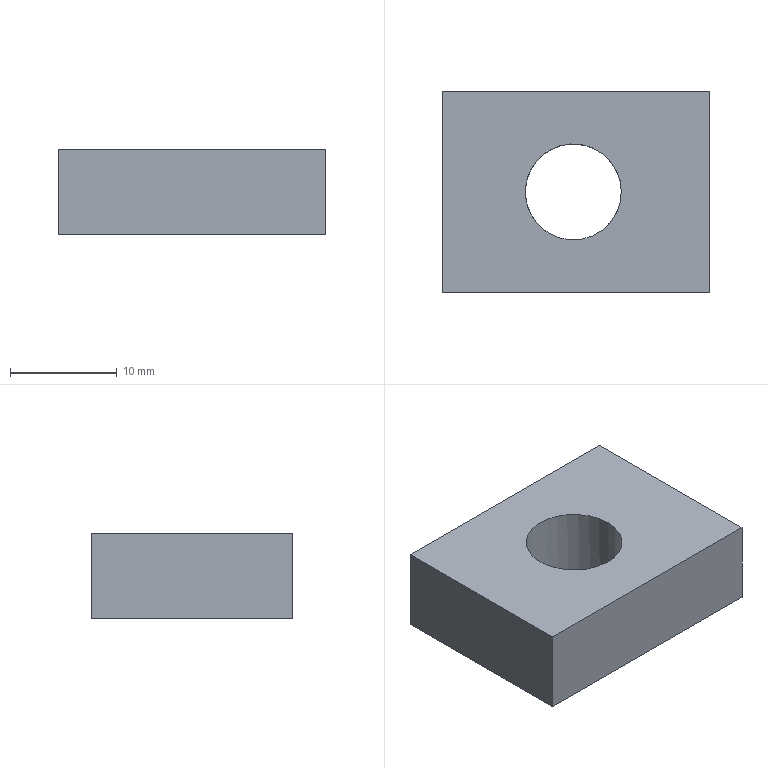Part | STEP file | gslz 2016.10.28-10_id1158_x_t | 1 solid | 7 faces | box 25.1 x 18.9 x 8 mm | volume 3286 mm3 | plane 6 | cylinder 1 | commonest cylinder face diameters 9 x1
STEP:
#1=CARTESIAN_POINT('',(0.,0.,0.));
#2=DIRECTION('',(0.,0.,1.));
#3=DIRECTION('',(1.,0.,0.));
#4=AXIS2_PLACEMENT_3D('',#1,#2,#3);
#5=CARTESIAN_POINT('',(-705.8,671.25,110.));
#6=VERTEX_POINT('',#5);
#7=CARTESIAN_POINT('',(-705.8,690.15,110.));
#8=VERTEX_POINT('',#7);
#9=CARTESIAN_POINT('',(-705.8,701.15,110.));
#10=DIRECTION('',(0.,1.,0.));
#11=VECTOR('',#10,1.);
#12=LINE('',#9,#11);
#13=CARTESIAN_POINT('',(-705.8,701.15,110.));
#14=DIRECTION('',(1.,0.,0.));
#15=DIRECTION('',(0.,0.,1.));
#16=AXIS2_PLACEMENT_3D('',#13,#14,#15);
#17=PLANE('',#16);
#18=CARTESIAN_POINT('',(0.,0.));
#19=DIRECTION('',(0.,-1.));
#20=VECTOR('',#19,1.);
#21=LINE('',#18,#20);
#22=(GEOMETRIC_REPRESENTATION_CONTEXT(2)PARAMETRIC_REPRESENTATION_CONTEXT()REPRESENTATION_CONTEXT('',''));
#23=DEFINITIONAL_REPRESENTATION('',(#21),#22);
#24=PCURVE('',#17,#23);
#25=CARTESIAN_POINT('',(-702.3,701.15,110.));
#26=DIRECTION('',(0.,0.,-1.));
#27=DIRECTION('',(1.,0.,0.));
#28=AXIS2_PLACEMENT_3D('',#25,#26,#27);
#29=PLANE('',#28);
#30=CARTESIAN_POINT('',(-3.5,0.));
#31=DIRECTION('',(0.,-1.));
#32=VECTOR('',#31,1.);
#33=LINE('',#30,#32);
#34=(GEOMETRIC_REPRESENTATION_CONTEXT(2)PARAMETRIC_REPRESENTATION_CONTEXT()REPRESENTATION_CONTEXT('',''));
#35=DEFINITIONAL_REPRESENTATION('',(#33),#34);
#36=PCURVE('',#29,#35);
#37=SURFACE_CURVE('',#12,(#24,#36),.PCURVE_S1.);
#38=EDGE_CURVE('',#6,#8,#37,.T.);
#39=ORIENTED_EDGE('',*,*,#38,.T.);
#40=CARTESIAN_POINT('',(-705.8,690.15,102.));
#41=VERTEX_POINT('',#40);
#42=CARTESIAN_POINT('',(-705.8,690.15,35.163));
#43=DIRECTION('',(0.,0.,-1.));
#44=VECTOR('',#43,1.);
#45=LINE('',#42,#44);
#46=CARTESIAN_POINT('',(-74.837,11.));
#47=DIRECTION('',(-1.,0.));
#48=VECTOR('',#47,1.);
#49=LINE('',#46,#48);
#50=(GEOMETRIC_REPRESENTATION_CONTEXT(2)PARAMETRIC_REPRESENTATION_CONTEXT()REPRESENTATION_CONTEXT('',''));
#51=DEFINITIONAL_REPRESENTATION('',(#49),#50);
#52=PCURVE('',#17,#51);
#53=CARTESIAN_POINT('',(-681.2,690.15,35.163));
#54=DIRECTION('',(0.,-1.,0.));
#55=DIRECTION('',(0.,0.,1.));
#56=AXIS2_PLACEMENT_3D('',#53,#54,#55);
#57=PLANE('',#56);
#58=CARTESIAN_POINT('',(0.,24.6));
#59=DIRECTION('',(-1.,0.));
#60=VECTOR('',#59,1.);
#61=LINE('',#58,#60);
#62=(GEOMETRIC_REPRESENTATION_CONTEXT(2)PARAMETRIC_REPRESENTATION_CONTEXT()REPRESENTATION_CONTEXT('',''));
#63=DEFINITIONAL_REPRESENTATION('',(#61),#62);
#64=PCURVE('',#57,#63);
#65=SURFACE_CURVE('',#45,(#52,#64),.PCURVE_S1.);
#66=EDGE_CURVE('',#8,#41,#65,.T.);
#67=ORIENTED_EDGE('',*,*,#66,.T.);
#68=CARTESIAN_POINT('',(-705.8,671.25,102.));
#69=VERTEX_POINT('',#68);
#70=CARTESIAN_POINT('',(-705.8,701.15,102.));
#71=DIRECTION('',(0.,1.,0.));
#72=VECTOR('',#71,1.);
#73=LINE('',#70,#72);
#74=CARTESIAN_POINT('',(-8.,0.));
#75=DIRECTION('',(0.,-1.));
#76=VECTOR('',#75,1.);
#77=LINE('',#74,#76);
#78=(GEOMETRIC_REPRESENTATION_CONTEXT(2)PARAMETRIC_REPRESENTATION_CONTEXT()REPRESENTATION_CONTEXT('',''));
#79=DEFINITIONAL_REPRESENTATION('',(#77),#78);
#80=PCURVE('',#17,#79);
#81=CARTESIAN_POINT('',(-703.8,701.15,102.));
#82=DIRECTION('',(0.,0.,1.));
#83=DIRECTION('',(-1.,0.,0.));
#84=AXIS2_PLACEMENT_3D('',#81,#82,#83);
#85=PLANE('',#84);
#86=CARTESIAN_POINT('',(2.,0.));
#87=DIRECTION('',(0.,-1.));
#88=VECTOR('',#87,1.);
#89=LINE('',#86,#88);
#90=(GEOMETRIC_REPRESENTATION_CONTEXT(2)PARAMETRIC_REPRESENTATION_CONTEXT()REPRESENTATION_CONTEXT('',''));
#91=DEFINITIONAL_REPRESENTATION('',(#89),#90);
#92=PCURVE('',#85,#91);
#93=SURFACE_CURVE('',#73,(#80,#92),.PCURVE_S1.);
#94=EDGE_CURVE('',#69,#41,#93,.T.);
#95=ORIENTED_EDGE('',*,*,#94,.F.);
#96=CARTESIAN_POINT('',(-705.8,671.25,35.163));
#97=DIRECTION('',(0.,0.,-1.));
#98=VECTOR('',#97,1.);
#99=LINE('',#96,#98);
#100=CARTESIAN_POINT('',(-74.837,29.9));
#101=DIRECTION('',(-1.,0.));
#102=VECTOR('',#101,1.);
#103=LINE('',#100,#102);
#104=(GEOMETRIC_REPRESENTATION_CONTEXT(2)PARAMETRIC_REPRESENTATION_CONTEXT()REPRESENTATION_CONTEXT('',''));
#105=DEFINITIONAL_REPRESENTATION('',(#103),#104);
#106=PCURVE('',#17,#105);
#107=CARTESIAN_POINT('',(-705.8,671.25,35.163));
#108=DIRECTION('',(0.,1.,0.));
#109=DIRECTION('',(0.,0.,-1.));
#110=AXIS2_PLACEMENT_3D('',#107,#108,#109);
#111=PLANE('',#110);
#112=CARTESIAN_POINT('',(0.,0.));
#113=DIRECTION('',(1.,0.));
#114=VECTOR('',#113,1.);
#115=LINE('',#112,#114);
#116=(GEOMETRIC_REPRESENTATION_CONTEXT(2)PARAMETRIC_REPRESENTATION_CONTEXT()REPRESENTATION_CONTEXT('',''));
#117=DEFINITIONAL_REPRESENTATION('',(#115),#116);
#118=PCURVE('',#111,#117);
#119=SURFACE_CURVE('',#99,(#106,#118),.PCURVE_S1.);
#120=EDGE_CURVE('',#6,#69,#119,.T.);
#121=ORIENTED_EDGE('',*,*,#120,.F.);
#122=EDGE_LOOP('',(#39,#67,#95,#121));
#123=FACE_BOUND('',#122,.T.);
#124=ADVANCED_FACE('',(#123),#17,.F.);
#125=CARTESIAN_POINT('',(-680.7,690.15,102.));
#126=VERTEX_POINT('',#125);
#127=CARTESIAN_POINT('',(-703.8,690.15,102.));
#128=DIRECTION('',(1.,0.,0.));
#129=VECTOR('',#128,1.);
#130=LINE('',#127,#129);
#131=CARTESIAN_POINT('',(0.,11.));
#132=DIRECTION('',(-1.,0.));
#133=VECTOR('',#132,1.);
#134=LINE('',#131,#133);
#135=(GEOMETRIC_REPRESENTATION_CONTEXT(2)PARAMETRIC_REPRESENTATION_CONTEXT()REPRESENTATION_CONTEXT('',''));
#136=DEFINITIONAL_REPRESENTATION('',(#134),#135);
#137=PCURVE('',#85,#136);
#138=CARTESIAN_POINT('',(66.837,22.6));
#139=DIRECTION('',(0.,-1.));
#140=VECTOR('',#139,1.);
#141=LINE('',#138,#140);
#142=(GEOMETRIC_REPRESENTATION_CONTEXT(2)PARAMETRIC_REPRESENTATION_CONTEXT()REPRESENTATION_CONTEXT('',''));
#143=DEFINITIONAL_REPRESENTATION('',(#141),#142);
#144=PCURVE('',#57,#143);
#145=SURFACE_CURVE('',#130,(#137,#144),.PCURVE_S1.);
#146=EDGE_CURVE('',#41,#126,#145,.T.);
#147=ORIENTED_EDGE('',*,*,#146,.T.);
#148=CARTESIAN_POINT('',(-680.7,671.25,102.));
#149=VERTEX_POINT('',#148);
#150=CARTESIAN_POINT('',(-680.7,701.15,102.));
#151=DIRECTION('',(0.,-1.,0.));
#152=VECTOR('',#151,1.);
#153=LINE('',#150,#152);
#154=CARTESIAN_POINT('',(-23.1,0.));
#155=DIRECTION('',(0.,1.));
#156=VECTOR('',#155,1.);
#157=LINE('',#154,#156);
#158=(GEOMETRIC_REPRESENTATION_CONTEXT(2)PARAMETRIC_REPRESENTATION_CONTEXT()REPRESENTATION_CONTEXT('',''));
#159=DEFINITIONAL_REPRESENTATION('',(#157),#158);
#160=PCURVE('',#85,#159);
#161=CARTESIAN_POINT('',(-680.7,701.15,106.));
#162=DIRECTION('',(-1.,0.,0.));
#163=DIRECTION('',(0.,0.,-1.));
#164=AXIS2_PLACEMENT_3D('',#161,#162,#163);
#165=PLANE('',#164);
#166=CARTESIAN_POINT('',(4.,0.));
#167=DIRECTION('',(0.,1.));
#168=VECTOR('',#167,1.);
#169=LINE('',#166,#168);
#170=(GEOMETRIC_REPRESENTATION_CONTEXT(2)PARAMETRIC_REPRESENTATION_CONTEXT()REPRESENTATION_CONTEXT('',''));
#171=DEFINITIONAL_REPRESENTATION('',(#169),#170);
#172=PCURVE('',#165,#171);
#173=SURFACE_CURVE('',#153,(#160,#172),.PCURVE_S1.);
#174=EDGE_CURVE('',#126,#149,#173,.T.);
#175=ORIENTED_EDGE('',*,*,#174,.T.);
#176=CARTESIAN_POINT('',(-703.8,671.25,102.));
#177=DIRECTION('',(-1.,0.,0.));
#178=VECTOR('',#177,1.);
#179=LINE('',#176,#178);
#180=CARTESIAN_POINT('',(0.,29.9));
#181=DIRECTION('',(1.,0.));
#182=VECTOR('',#181,1.);
#183=LINE('',#180,#182);
#184=(GEOMETRIC_REPRESENTATION_CONTEXT(2)PARAMETRIC_REPRESENTATION_CONTEXT()REPRESENTATION_CONTEXT('',''));
#185=DEFINITIONAL_REPRESENTATION('',(#183),#184);
#186=PCURVE('',#85,#185);
#187=CARTESIAN_POINT('',(-66.837,-2.));
#188=DIRECTION('',(0.,1.));
#189=VECTOR('',#188,1.);
#190=LINE('',#187,#189);
#191=(GEOMETRIC_REPRESENTATION_CONTEXT(2)PARAMETRIC_REPRESENTATION_CONTEXT()REPRESENTATION_CONTEXT('',''));
#192=DEFINITIONAL_REPRESENTATION('',(#190),#191);
#193=PCURVE('',#111,#192);
#194=SURFACE_CURVE('',#179,(#186,#193),.PCURVE_S1.);
#195=EDGE_CURVE('',#149,#69,#194,.T.);
#196=ORIENTED_EDGE('',*,*,#195,.T.);
#197=ORIENTED_EDGE('',*,*,#94,.T.);
#198=EDGE_LOOP('',(#147,#175,#196,#197));
#199=FACE_BOUND('',#198,.T.);
#200=CARTESIAN_POINT('',(-698.,680.7,102.));
#201=VERTEX_POINT('',#200);
#202=CARTESIAN_POINT('',(-689.,680.7,102.));
#203=VERTEX_POINT('',#202);
#204=CARTESIAN_POINT('',(-693.5,680.7,102.));
#205=DIRECTION('',(0.,0.,1.));
#206=DIRECTION('',(-1.,0.,0.));
#207=AXIS2_PLACEMENT_3D('',#204,#205,#206);
#208=CIRCLE('',#207,4.5);
#209=CARTESIAN_POINT('',(-10.3,20.45));
#210=DIRECTION('',(1.,0.));
#211=AXIS2_PLACEMENT_2D('',#209,#210);
#212=CIRCLE('',#211,4.5);
#213=(GEOMETRIC_REPRESENTATION_CONTEXT(2)PARAMETRIC_REPRESENTATION_CONTEXT()REPRESENTATION_CONTEXT('',''));
#214=DEFINITIONAL_REPRESENTATION('',(#212),#213);
#215=PCURVE('',#85,#214);
#216=CARTESIAN_POINT('',(-693.5,680.7,219.073));
#217=DIRECTION('',(0.,0.,-1.));
#218=DIRECTION('',(1.,0.,0.));
#219=AXIS2_PLACEMENT_3D('',#216,#217,#218);
#220=CYLINDRICAL_SURFACE('',#219,4.5);
#221=CARTESIAN_POINT('',(3.142,117.073));
#222=DIRECTION('',(-1.,0.));
#223=VECTOR('',#222,1.);
#224=LINE('',#221,#223);
#225=(GEOMETRIC_REPRESENTATION_CONTEXT(2)PARAMETRIC_REPRESENTATION_CONTEXT()REPRESENTATION_CONTEXT('',''));
#226=DEFINITIONAL_REPRESENTATION('',(#224),#225);
#227=PCURVE('',#220,#226);
#228=SURFACE_CURVE('',#208,(#215,#227),.PCURVE_S1.);
#229=EDGE_CURVE('',#201,#203,#228,.T.);
#230=ORIENTED_EDGE('',*,*,#229,.T.);
#231=CARTESIAN_POINT('',(-693.5,680.7,102.));
#232=DIRECTION('',(0.,0.,1.));
#233=DIRECTION('',(-1.,0.,0.));
#234=AXIS2_PLACEMENT_3D('',#231,#232,#233);
#235=CIRCLE('',#234,4.5);
#236=CARTESIAN_POINT('',(-10.3,20.45));
#237=DIRECTION('',(1.,0.));
#238=AXIS2_PLACEMENT_2D('',#236,#237);
#239=CIRCLE('',#238,4.5);
#240=(GEOMETRIC_REPRESENTATION_CONTEXT(2)PARAMETRIC_REPRESENTATION_CONTEXT()REPRESENTATION_CONTEXT('',''));
#241=DEFINITIONAL_REPRESENTATION('',(#239),#240);
#242=PCURVE('',#85,#241);
#243=CARTESIAN_POINT('',(9.425,117.073));
#244=DIRECTION('',(-1.,0.));
#245=VECTOR('',#244,1.);
#246=LINE('',#243,#245);
#247=(GEOMETRIC_REPRESENTATION_CONTEXT(2)PARAMETRIC_REPRESENTATION_CONTEXT()REPRESENTATION_CONTEXT('',''));
#248=DEFINITIONAL_REPRESENTATION('',(#246),#247);
#249=PCURVE('',#220,#248);
#250=SURFACE_CURVE('',#235,(#242,#249),.PCURVE_S1.);
#251=EDGE_CURVE('',#203,#201,#250,.T.);
#252=ORIENTED_EDGE('',*,*,#251,.T.);
#253=EDGE_LOOP('',(#230,#252));
#254=FACE_BOUND('',#253,.T.);
#255=ADVANCED_FACE('',(#199,#254),#85,.F.);
#256=CARTESIAN_POINT('',(-680.7,690.15,110.));
#257=VERTEX_POINT('',#256);
#258=CARTESIAN_POINT('',(-702.3,690.15,110.));
#259=DIRECTION('',(-1.,0.,0.));
#260=VECTOR('',#259,1.);
#261=LINE('',#258,#260);
#262=CARTESIAN_POINT('',(0.,11.));
#263=DIRECTION('',(-1.,0.));
#264=VECTOR('',#263,1.);
#265=LINE('',#262,#264);
#266=(GEOMETRIC_REPRESENTATION_CONTEXT(2)PARAMETRIC_REPRESENTATION_CONTEXT()REPRESENTATION_CONTEXT('',''));
#267=DEFINITIONAL_REPRESENTATION('',(#265),#266);
#268=PCURVE('',#29,#267);
#269=CARTESIAN_POINT('',(74.837,21.1));
#270=DIRECTION('',(0.,1.));
#271=VECTOR('',#270,1.);
#272=LINE('',#269,#271);
#273=(GEOMETRIC_REPRESENTATION_CONTEXT(2)PARAMETRIC_REPRESENTATION_CONTEXT()REPRESENTATION_CONTEXT('',''));
#274=DEFINITIONAL_REPRESENTATION('',(#272),#273);
#275=PCURVE('',#57,#274);
#276=SURFACE_CURVE('',#261,(#268,#275),.PCURVE_S1.);
#277=EDGE_CURVE('',#257,#8,#276,.T.);
#278=ORIENTED_EDGE('',*,*,#277,.T.);
#279=ORIENTED_EDGE('',*,*,#38,.F.);
#280=CARTESIAN_POINT('',(-680.7,671.25,110.));
#281=VERTEX_POINT('',#280);
#282=CARTESIAN_POINT('',(-702.3,671.25,110.));
#283=DIRECTION('',(1.,0.,0.));
#284=VECTOR('',#283,1.);
#285=LINE('',#282,#284);
#286=CARTESIAN_POINT('',(0.,29.9));
#287=DIRECTION('',(1.,0.));
#288=VECTOR('',#287,1.);
#289=LINE('',#286,#288);
#290=(GEOMETRIC_REPRESENTATION_CONTEXT(2)PARAMETRIC_REPRESENTATION_CONTEXT()REPRESENTATION_CONTEXT('',''));
#291=DEFINITIONAL_REPRESENTATION('',(#289),#290);
#292=PCURVE('',#29,#291);
#293=CARTESIAN_POINT('',(-74.837,-3.5));
#294=DIRECTION('',(0.,-1.));
#295=VECTOR('',#294,1.);
#296=LINE('',#293,#295);
#297=(GEOMETRIC_REPRESENTATION_CONTEXT(2)PARAMETRIC_REPRESENTATION_CONTEXT()REPRESENTATION_CONTEXT('',''));
#298=DEFINITIONAL_REPRESENTATION('',(#296),#297);
#299=PCURVE('',#111,#298);
#300=SURFACE_CURVE('',#285,(#292,#299),.PCURVE_S1.);
#301=EDGE_CURVE('',#6,#281,#300,.T.);
#302=ORIENTED_EDGE('',*,*,#301,.T.);
#303=CARTESIAN_POINT('',(-680.7,701.15,110.));
#304=DIRECTION('',(0.,1.,0.));
#305=VECTOR('',#304,1.);
#306=LINE('',#303,#305);
#307=CARTESIAN_POINT('',(21.6,0.));
#308=DIRECTION('',(0.,-1.));
#309=VECTOR('',#308,1.);
#310=LINE('',#307,#309);
#311=(GEOMETRIC_REPRESENTATION_CONTEXT(2)PARAMETRIC_REPRESENTATION_CONTEXT()REPRESENTATION_CONTEXT('',''));
#312=DEFINITIONAL_REPRESENTATION('',(#310),#311);
#313=PCURVE('',#29,#312);
#314=CARTESIAN_POINT('',(-4.,0.));
#315=DIRECTION('',(0.,-1.));
#316=VECTOR('',#315,1.);
#317=LINE('',#314,#316);
#318=(GEOMETRIC_REPRESENTATION_CONTEXT(2)PARAMETRIC_REPRESENTATION_CONTEXT()REPRESENTATION_CONTEXT('',''));
#319=DEFINITIONAL_REPRESENTATION('',(#317),#318);
#320=PCURVE('',#165,#319);
#321=SURFACE_CURVE('',#306,(#313,#320),.PCURVE_S1.);
#322=EDGE_CURVE('',#281,#257,#321,.T.);
#323=ORIENTED_EDGE('',*,*,#322,.T.);
#324=EDGE_LOOP('',(#278,#279,#302,#323));
#325=FACE_BOUND('',#324,.T.);
#326=CARTESIAN_POINT('',(-689.,680.7,110.));
#327=VERTEX_POINT('',#326);
#328=CARTESIAN_POINT('',(-693.5,680.7,110.));
#329=DIRECTION('',(0.,0.,1.));
#330=DIRECTION('',(1.,0.,0.));
#331=AXIS2_PLACEMENT_3D('',#328,#329,#330);
#332=CIRCLE('',#331,4.5);
#333=CARTESIAN_POINT('',(13.3,20.45));
#334=CARTESIAN_POINT('',(13.3,12.656));
#335=CARTESIAN_POINT('',(6.55,16.553));
#336=CARTESIAN_POINT('',(-0.2,20.45));
#337=CARTESIAN_POINT('',(6.55,24.347));
#338=CARTESIAN_POINT('',(13.3,28.244));
#339=CARTESIAN_POINT('',(13.3,20.45));
#340=(BOUNDED_CURVE()B_SPLINE_CURVE(2,(#333,#334,#335,#336,#337,#338,#339),.UNSPECIFIED.,.T.,.F.)B_SPLINE_CURVE_WITH_KNOTS((1,2,2,2,2,1),(-2.094,0.,2.094,4.189,6.283,8.378),.UNSPECIFIED.)CURVE()GEOMETRIC_REPRESENTATION_ITEM()RATIONAL_B_SPLINE_CURVE((1.,0.5,1.,0.5,1.,0.5,1.))REPRESENTATION_ITEM(''));
#341=(GEOMETRIC_REPRESENTATION_CONTEXT(2)PARAMETRIC_REPRESENTATION_CONTEXT()REPRESENTATION_CONTEXT('',''));
#342=DEFINITIONAL_REPRESENTATION('',(#340),#341);
#343=PCURVE('',#29,#342);
#344=CARTESIAN_POINT('',(6.283,109.073));
#345=DIRECTION('',(-1.,0.));
#346=VECTOR('',#345,1.);
#347=LINE('',#344,#346);
#348=(GEOMETRIC_REPRESENTATION_CONTEXT(2)PARAMETRIC_REPRESENTATION_CONTEXT()REPRESENTATION_CONTEXT('',''));
#349=DEFINITIONAL_REPRESENTATION('',(#347),#348);
#350=PCURVE('',#220,#349);
#351=SURFACE_CURVE('',#332,(#343,#350),.PCURVE_S1.);
#352=EDGE_CURVE('',#327,#327,#351,.T.);
#353=ORIENTED_EDGE('',*,*,#352,.F.);
#354=EDGE_LOOP('',(#353));
#355=FACE_BOUND('',#354,.T.);
#356=ADVANCED_FACE('',(#325,#355),#29,.F.);
#357=ORIENTED_EDGE('',*,*,#229,.T.);
#358=CARTESIAN_POINT('',(-689.,680.7,110.));
#359=CARTESIAN_POINT('',(-689.,680.7,102.));
#360=B_SPLINE_CURVE_WITH_KNOTS('',1,(#358,#359),.UNSPECIFIED.,.F.,.F.,(2,2),(109.073,117.073),.PIECEWISE_BEZIER_KNOTS.);
#361=CARTESIAN_POINT('',(0.,0.));
#362=DIRECTION('',(0.,1.));
#363=VECTOR('',#362,1.);
#364=LINE('',#361,#363);
#365=(GEOMETRIC_REPRESENTATION_CONTEXT(2)PARAMETRIC_REPRESENTATION_CONTEXT()REPRESENTATION_CONTEXT('',''));
#366=DEFINITIONAL_REPRESENTATION('',(#364),#365);
#367=PCURVE('',#220,#366);
#368=CARTESIAN_POINT('',(6.283,0.));
#369=DIRECTION('',(0.,1.));
#370=VECTOR('',#369,1.);
#371=LINE('',#368,#370);
#372=(GEOMETRIC_REPRESENTATION_CONTEXT(2)PARAMETRIC_REPRESENTATION_CONTEXT()REPRESENTATION_CONTEXT('',''));
#373=DEFINITIONAL_REPRESENTATION('',(#371),#372);
#374=PCURVE('',#220,#373);
#375=SEAM_CURVE('',#360,(#367,#374),.PCURVE_S1.);
#376=EDGE_CURVE('',#327,#203,#375,.T.);
#377=ORIENTED_EDGE('',*,*,#376,.F.);
#378=ORIENTED_EDGE('',*,*,#352,.F.);
#379=ORIENTED_EDGE('',*,*,#376,.T.);
#380=ORIENTED_EDGE('',*,*,#251,.T.);
#381=EDGE_LOOP('',(#357,#377,#378,#379,#380));
#382=FACE_BOUND('',#381,.F.);
#383=ADVANCED_FACE('',(#382),#220,.F.);
#384=CARTESIAN_POINT('',(-680.7,690.15,35.163));
#385=DIRECTION('',(0.,0.,-1.));
#386=VECTOR('',#385,1.);
#387=LINE('',#384,#386);
#388=CARTESIAN_POINT('',(70.837,11.));
#389=DIRECTION('',(1.,0.));
#390=VECTOR('',#389,1.);
#391=LINE('',#388,#390);
#392=(GEOMETRIC_REPRESENTATION_CONTEXT(2)PARAMETRIC_REPRESENTATION_CONTEXT()REPRESENTATION_CONTEXT('',''));
#393=DEFINITIONAL_REPRESENTATION('',(#391),#392);
#394=PCURVE('',#165,#393);
#395=CARTESIAN_POINT('',(0.,-0.5));
#396=DIRECTION('',(-1.,0.));
#397=VECTOR('',#396,1.);
#398=LINE('',#395,#397);
#399=(GEOMETRIC_REPRESENTATION_CONTEXT(2)PARAMETRIC_REPRESENTATION_CONTEXT()REPRESENTATION_CONTEXT('',''));
#400=DEFINITIONAL_REPRESENTATION('',(#398),#399);
#401=PCURVE('',#57,#400);
#402=SURFACE_CURVE('',#387,(#394,#401),.PCURVE_S1.);
#403=EDGE_CURVE('',#257,#126,#402,.T.);
#404=ORIENTED_EDGE('',*,*,#403,.F.);
#405=ORIENTED_EDGE('',*,*,#322,.F.);
#406=CARTESIAN_POINT('',(-680.7,671.25,106.));
#407=DIRECTION('',(0.,0.,-1.));
#408=VECTOR('',#407,1.);
#409=LINE('',#406,#408);
#410=CARTESIAN_POINT('',(0.,29.9));
#411=DIRECTION('',(1.,0.));
#412=VECTOR('',#411,1.);
#413=LINE('',#410,#412);
#414=(GEOMETRIC_REPRESENTATION_CONTEXT(2)PARAMETRIC_REPRESENTATION_CONTEXT()REPRESENTATION_CONTEXT('',''));
#415=DEFINITIONAL_REPRESENTATION('',(#413),#414);
#416=PCURVE('',#165,#415);
#417=CARTESIAN_POINT('',(-70.837,-25.1));
#418=DIRECTION('',(1.,0.));
#419=VECTOR('',#418,1.);
#420=LINE('',#417,#419);
#421=(GEOMETRIC_REPRESENTATION_CONTEXT(2)PARAMETRIC_REPRESENTATION_CONTEXT()REPRESENTATION_CONTEXT('',''));
#422=DEFINITIONAL_REPRESENTATION('',(#420),#421);
#423=PCURVE('',#111,#422);
#424=SURFACE_CURVE('',#409,(#416,#423),.PCURVE_S1.);
#425=EDGE_CURVE('',#281,#149,#424,.T.);
#426=ORIENTED_EDGE('',*,*,#425,.T.);
#427=ORIENTED_EDGE('',*,*,#174,.F.);
#428=EDGE_LOOP('',(#404,#405,#426,#427));
#429=FACE_BOUND('',#428,.T.);
#430=ADVANCED_FACE('',(#429),#165,.F.);
#431=ORIENTED_EDGE('',*,*,#301,.F.);
#432=ORIENTED_EDGE('',*,*,#120,.T.);
#433=ORIENTED_EDGE('',*,*,#195,.F.);
#434=ORIENTED_EDGE('',*,*,#425,.F.);
#435=EDGE_LOOP('',(#431,#432,#433,#434));
#436=FACE_BOUND('',#435,.T.);
#437=ADVANCED_FACE('',(#436),#111,.F.);
#438=ORIENTED_EDGE('',*,*,#403,.T.);
#439=ORIENTED_EDGE('',*,*,#146,.F.);
#440=ORIENTED_EDGE('',*,*,#66,.F.);
#441=ORIENTED_EDGE('',*,*,#277,.F.);
#442=EDGE_LOOP('',(#438,#439,#440,#441));
#443=FACE_BOUND('',#442,.T.);
#444=ADVANCED_FACE('',(#443),#57,.F.);
#445=CLOSED_SHELL('',(#124,#255,#356,#383,#430,#437,#444));
#446=MANIFOLD_SOLID_BREP('',#445);
#447=(LENGTH_UNIT()NAMED_UNIT(*)SI_UNIT(.MILLI.,.METRE.));
#448=UNCERTAINTY_MEASURE_WITH_UNIT(LENGTH_MEASURE(0.000002),#447,'','');
#449=(NAMED_UNIT(*)PLANE_ANGLE_UNIT()SI_UNIT($,.RADIAN.));
#450=(NAMED_UNIT(*)SI_UNIT($,.STERADIAN.)SOLID_ANGLE_UNIT());
#451=(GEOMETRIC_REPRESENTATION_CONTEXT(3)GLOBAL_UNCERTAINTY_ASSIGNED_CONTEXT((#448))GLOBAL_UNIT_ASSIGNED_CONTEXT((#447,#449,#450))REPRESENTATION_CONTEXT('',''));
#452=ADVANCED_BREP_SHAPE_REPRESENTATION('',(#4,#446),#451);